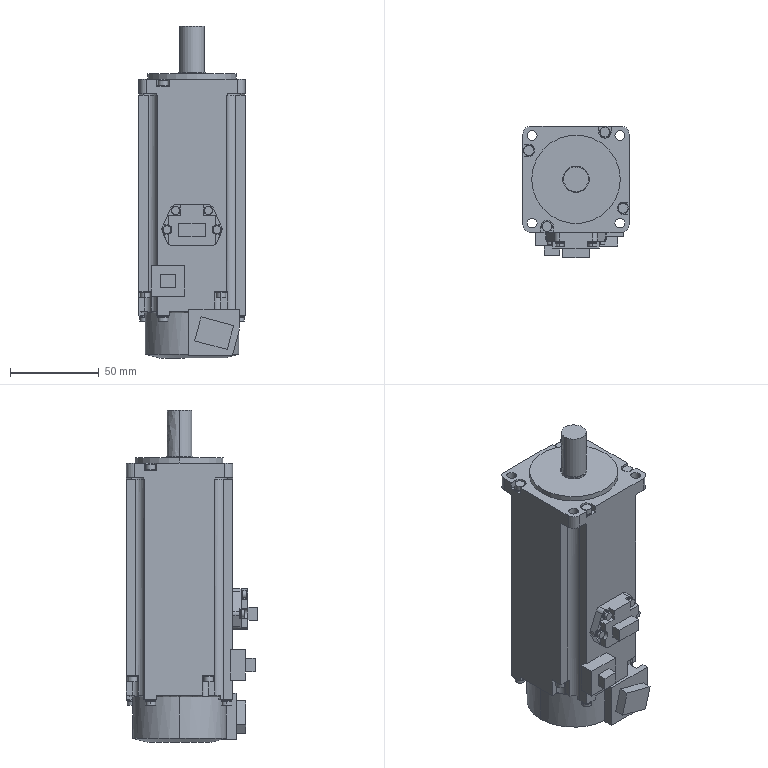Part | SolidWorks | features BaseBody 1 | 1 solid | 331 faces | box 60 x 74.2 x 187.5 mm | volume 503412 mm3 | plane 187 | cylinder 134 | spline 9 | cone 1 | commonest cylinder face diameters 5.5 x32 6 x30 7 x16 4.5 x8 4.8 x8 5 x8